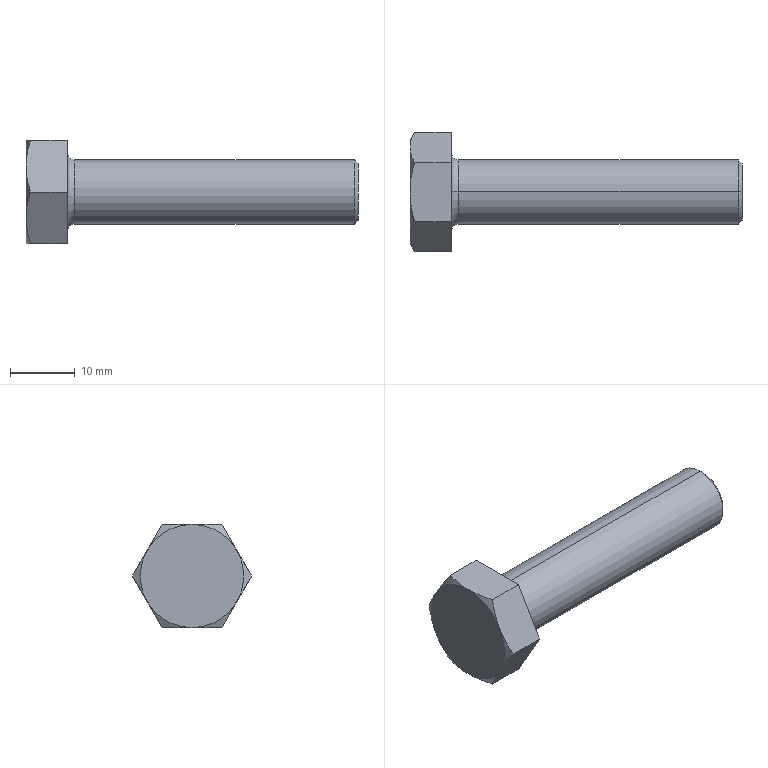Part | SolidWorks | features Chamfer 2, RevCut 2, Revolution 2, Extrusion 1, ICE 1 | 1 solid | 21 faces | box 51.4 x 18.475 x 16 mm | volume 4953 mm3 | plane 9 | cone 8 | cylinder 2 | torus 2 | commonest cylinder face diameters 10 x2
STEP:
#1=CARTESIAN_POINT('',(51.4,0.,-4.444));
#2=VERTEX_POINT('',#1);
#3=CARTESIAN_POINT('',(51.4,0.,4.444));
#4=VERTEX_POINT('',#3);
#5=CARTESIAN_POINT('',(51.4,0.,0.));
#6=DIRECTION('',(1.,0.,0.));
#7=DIRECTION('',(0.,0.,1.));
#8=AXIS2_PLACEMENT_3D('',#5,#6,#7);
#9=CIRCLE('',#8,4.444);
#10=EDGE_CURVE('',#2,#4,#9,.T.);
#11=ORIENTED_EDGE('',*,*,#10,.F.);
#12=CARTESIAN_POINT('',(50.844,0.,-5.));
#13=VERTEX_POINT('',#12);
#14=CARTESIAN_POINT('',(50.844,0.,-5.));
#15=DIRECTION('',(-0.7071,0.,-0.7071));
#16=VECTOR('',#15,1000.);
#17=LINE('',#14,#16);
#18=EDGE_CURVE('',#2,#13,#17,.T.);
#19=ORIENTED_EDGE('',*,*,#18,.T.);
#20=CARTESIAN_POINT('',(50.844,0.,5.));
#21=VERTEX_POINT('',#20);
#22=CARTESIAN_POINT('',(50.844,0.,0.));
#23=DIRECTION('',(-1.,0.,0.));
#24=DIRECTION('',(0.,0.,1.));
#25=AXIS2_PLACEMENT_3D('',#22,#23,#24);
#26=CIRCLE('',#25,5.);
#27=EDGE_CURVE('',#21,#13,#26,.T.);
#28=ORIENTED_EDGE('',*,*,#27,.F.);
#29=CARTESIAN_POINT('',(50.844,0.,5.));
#30=DIRECTION('',(-0.7071,0.,0.7071));
#31=VECTOR('',#30,1000.);
#32=LINE('',#29,#31);
#33=EDGE_CURVE('',#4,#21,#32,.T.);
#34=ORIENTED_EDGE('',*,*,#33,.F.);
#35=EDGE_LOOP('',(#11,#19,#28,#34));
#36=FACE_OUTER_BOUND('',#35,.T.);
#37=CARTESIAN_POINT('',(50.844,0.,0.));
#38=DIRECTION('',(-1.,0.,0.));
#39=DIRECTION('',(0.,0.,1.));
#40=AXIS2_PLACEMENT_3D('',#37,#38,#39);
#41=CONICAL_SURFACE('',#40,5.,0.7854);
#42=ADVANCED_FACE('',(#36),#41,.T.);
#43=ORIENTED_EDGE('',*,*,#27,.T.);
#44=CARTESIAN_POINT('',(7.5,0.,-5.));
#45=VERTEX_POINT('',#44);
#46=CARTESIAN_POINT('',(6.4,0.,-5.));
#47=DIRECTION('',(-1.,0.,0.));
#48=VECTOR('',#47,1000.);
#49=LINE('',#46,#48);
#50=EDGE_CURVE('',#13,#45,#49,.T.);
#51=ORIENTED_EDGE('',*,*,#50,.T.);
#52=CARTESIAN_POINT('',(7.5,0.,5.));
#53=VERTEX_POINT('',#52);
#54=CARTESIAN_POINT('',(7.5,0.,0.));
#55=DIRECTION('',(-1.,0.,0.));
#56=DIRECTION('',(0.,0.,1.));
#57=AXIS2_PLACEMENT_3D('',#54,#55,#56);
#58=CIRCLE('',#57,5.);
#59=EDGE_CURVE('',#53,#45,#58,.T.);
#60=ORIENTED_EDGE('',*,*,#59,.F.);
#61=CARTESIAN_POINT('',(6.4,0.,5.));
#62=DIRECTION('',(-1.,0.,0.));
#63=VECTOR('',#62,1000.);
#64=LINE('',#61,#63);
#65=EDGE_CURVE('',#21,#53,#64,.T.);
#66=ORIENTED_EDGE('',*,*,#65,.F.);
#67=EDGE_LOOP('',(#43,#51,#60,#66));
#68=FACE_OUTER_BOUND('',#67,.T.);
#69=CARTESIAN_POINT('',(6.4,0.,0.));
#70=DIRECTION('',(-1.,0.,0.));
#71=DIRECTION('',(0.,0.,1.));
#72=AXIS2_PLACEMENT_3D('',#69,#70,#71);
#73=CYLINDRICAL_SURFACE('',#72,5.);
#74=ADVANCED_FACE('',(#68),#73,.T.);
#75=CARTESIAN_POINT('',(6.4,0.,-6.1));
#76=VERTEX_POINT('',#75);
#77=CARTESIAN_POINT('',(6.4,0.,6.1));
#78=VERTEX_POINT('',#77);
#79=CARTESIAN_POINT('',(6.4,0.,0.));
#80=DIRECTION('',(-1.,0.,0.));
#81=DIRECTION('',(0.,0.,1.));
#82=AXIS2_PLACEMENT_3D('',#79,#80,#81);
#83=CIRCLE('',#82,6.1);
#84=EDGE_CURVE('',#76,#78,#83,.T.);
#85=ORIENTED_EDGE('',*,*,#84,.F.);
#86=CARTESIAN_POINT('',(7.5,0.,-6.1));
#87=DIRECTION('',(0.,1.,0.));
#88=DIRECTION('',(0.,0.,1.));
#89=AXIS2_PLACEMENT_3D('',#86,#87,#88);
#90=CIRCLE('',#89,1.1);
#91=EDGE_CURVE('',#76,#45,#90,.T.);
#92=ORIENTED_EDGE('',*,*,#91,.T.);
#93=CARTESIAN_POINT('',(7.5,0.,0.));
#94=DIRECTION('',(-1.,0.,0.));
#95=DIRECTION('',(0.,0.,1.));
#96=AXIS2_PLACEMENT_3D('',#93,#94,#95);
#97=CIRCLE('',#96,5.);
#98=EDGE_CURVE('',#45,#53,#97,.T.);
#99=ORIENTED_EDGE('',*,*,#98,.T.);
#100=CARTESIAN_POINT('',(7.5,0.,6.1));
#101=DIRECTION('',(0.,-1.,0.));
#102=DIRECTION('',(0.,0.,-1.));
#103=AXIS2_PLACEMENT_3D('',#100,#101,#102);
#104=CIRCLE('',#103,1.1);
#105=EDGE_CURVE('',#78,#53,#104,.T.);
#106=ORIENTED_EDGE('',*,*,#105,.F.);
#107=EDGE_LOOP('',(#85,#92,#99,#106));
#108=FACE_OUTER_BOUND('',#107,.T.);
#109=CARTESIAN_POINT('',(7.5,0.,0.));
#110=DIRECTION('',(-1.,0.,0.));
#111=DIRECTION('',(0.,0.,1.));
#112=AXIS2_PLACEMENT_3D('',#109,#110,#111);
#113=TOROIDAL_SURFACE('',#112,6.1,1.1);
#114=ADVANCED_FACE('',(#108),#113,.F.);
#115=CARTESIAN_POINT('',(6.4,-4.619,-8.));
#116=VERTEX_POINT('',#115);
#117=CARTESIAN_POINT('',(6.4,4.619,-8.));
#118=VERTEX_POINT('',#117);
#119=CARTESIAN_POINT('',(6.4,-4.619,-8.));
#120=DIRECTION('',(0.,1.,0.));
#121=VECTOR('',#120,1000.);
#122=LINE('',#119,#121);
#123=EDGE_CURVE('',#116,#118,#122,.T.);
#124=ORIENTED_EDGE('',*,*,#123,.T.);
#125=CARTESIAN_POINT('',(6.4,9.238,0.));
#126=VERTEX_POINT('',#125);
#127=CARTESIAN_POINT('',(6.4,4.619,-8.));
#128=DIRECTION('',(0.,0.5,0.866));
#129=VECTOR('',#128,1000.);
#130=LINE('',#127,#129);
#131=EDGE_CURVE('',#118,#126,#130,.T.);
#132=ORIENTED_EDGE('',*,*,#131,.T.);
#133=CARTESIAN_POINT('',(6.4,4.619,8.));
#134=VERTEX_POINT('',#133);
#135=CARTESIAN_POINT('',(6.4,9.238,0.));
#136=DIRECTION('',(0.,-0.5,0.866));
#137=VECTOR('',#136,1000.);
#138=LINE('',#135,#137);
#139=EDGE_CURVE('',#126,#134,#138,.T.);
#140=ORIENTED_EDGE('',*,*,#139,.T.);
#141=CARTESIAN_POINT('',(6.4,-4.619,8.));
#142=VERTEX_POINT('',#141);
#143=CARTESIAN_POINT('',(6.4,4.619,8.));
#144=DIRECTION('',(0.,-1.,0.));
#145=VECTOR('',#144,1000.);
#146=LINE('',#143,#145);
#147=EDGE_CURVE('',#134,#142,#146,.T.);
#148=ORIENTED_EDGE('',*,*,#147,.T.);
#149=CARTESIAN_POINT('',(6.4,-9.238,0.));
#150=VERTEX_POINT('',#149);
#151=CARTESIAN_POINT('',(6.4,-4.619,8.));
#152=DIRECTION('',(0.,-0.5,-0.866));
#153=VECTOR('',#152,1000.);
#154=LINE('',#151,#153);
#155=EDGE_CURVE('',#142,#150,#154,.T.);
#156=ORIENTED_EDGE('',*,*,#155,.T.);
#157=CARTESIAN_POINT('',(6.4,-9.238,0.));
#158=DIRECTION('',(0.,0.5,-0.866));
#159=VECTOR('',#158,1000.);
#160=LINE('',#157,#159);
#161=EDGE_CURVE('',#150,#116,#160,.T.);
#162=ORIENTED_EDGE('',*,*,#161,.T.);
#163=EDGE_LOOP('',(#124,#132,#140,#148,#156,#162));
#164=FACE_OUTER_BOUND('',#163,.T.);
#165=CARTESIAN_POINT('',(6.4,0.,0.));
#166=DIRECTION('',(-1.,0.,0.));
#167=DIRECTION('',(0.,0.,1.));
#168=AXIS2_PLACEMENT_3D('',#165,#166,#167);
#169=CIRCLE('',#168,6.1);
#170=EDGE_CURVE('',#78,#76,#169,.T.);
#171=ORIENTED_EDGE('',*,*,#170,.T.);
#172=ORIENTED_EDGE('',*,*,#84,.T.);
#173=EDGE_LOOP('',(#171,#172));
#174=FACE_BOUND('',#173,.T.);
#175=CARTESIAN_POINT('',(6.4,4.619,-8.));
#176=DIRECTION('',(1.,0.,0.));
#177=DIRECTION('',(0.,0.,-1.));
#178=AXIS2_PLACEMENT_3D('',#175,#176,#177);
#179=PLANE('',#178);
#180=ADVANCED_FACE('',(#164,#174),#179,.T.);
#181=CARTESIAN_POINT('',(0.7145,4.619,-8.));
#182=VERTEX_POINT('',#181);
#183=CARTESIAN_POINT('',(0.,0.,-8.));
#184=VERTEX_POINT('',#183);
#185=CARTESIAN_POINT('',(0.7145,4.619,-8.));
#186=CARTESIAN_POINT('',(0.4989,3.872,-8.));
#187=CARTESIAN_POINT('',(0.3194,3.115,-8.));
#188=CARTESIAN_POINT('',(0.06895,1.573,-8.));
#189=CARTESIAN_POINT('',(0.,0.781,-8.));
#190=CARTESIAN_POINT('',(0.,0.,-8.));
#191=B_SPLINE_CURVE_WITH_KNOTS('',3,(#185,#186,#187,#188,#189,#190),.UNSPECIFIED.,.F.,.F.,(4,2,4),(0.003372,0.005703,0.008035),.UNSPECIFIED.);
#192=EDGE_CURVE('',#182,#184,#191,.T.);
#193=ORIENTED_EDGE('',*,*,#192,.F.);
#194=CARTESIAN_POINT('',(6.4,4.619,-8.));
#195=DIRECTION('',(-1.,0.,0.));
#196=VECTOR('',#195,1000.);
#197=LINE('',#194,#196);
#198=EDGE_CURVE('',#118,#182,#197,.T.);
#199=ORIENTED_EDGE('',*,*,#198,.F.);
#200=ORIENTED_EDGE('',*,*,#123,.F.);
#201=CARTESIAN_POINT('',(0.7145,-4.619,-8.));
#202=VERTEX_POINT('',#201);
#203=CARTESIAN_POINT('',(6.4,-4.619,-8.));
#204=DIRECTION('',(-1.,0.,0.));
#205=VECTOR('',#204,1000.);
#206=LINE('',#203,#205);
#207=EDGE_CURVE('',#116,#202,#206,.T.);
#208=ORIENTED_EDGE('',*,*,#207,.T.);
#209=CARTESIAN_POINT('',(0.,0.,-8.));
#210=CARTESIAN_POINT('',(0.,-0.7805,-8.));
#211=CARTESIAN_POINT('',(0.06709,-1.556,-8.));
#212=CARTESIAN_POINT('',(0.3158,-3.098,-8.));
#213=CARTESIAN_POINT('',(0.4977,-3.868,-8.));
#214=CARTESIAN_POINT('',(0.7145,-4.619,-8.));
#215=B_SPLINE_CURVE_WITH_KNOTS('',3,(#209,#210,#211,#212,#213,#214),.UNSPECIFIED.,.F.,.F.,(4,2,4),(0.008035,0.01037,0.0127),.UNSPECIFIED.);
#216=EDGE_CURVE('',#184,#202,#215,.T.);
#217=ORIENTED_EDGE('',*,*,#216,.F.);
#218=EDGE_LOOP('',(#193,#199,#200,#208,#217));
#219=FACE_OUTER_BOUND('',#218,.T.);
#220=CARTESIAN_POINT('',(6.4,-4.619,-8.));
#221=DIRECTION('',(0.,0.,1.));
#222=DIRECTION('',(1.,0.,0.));
#223=AXIS2_PLACEMENT_3D('',#220,#221,#222);
#224=PLANE('',#223);
#225=ADVANCED_FACE('',(#219),#224,.F.);
#226=CARTESIAN_POINT('',(0.7145,9.238,0.));
#227=VERTEX_POINT('',#226);
#228=CARTESIAN_POINT('',(0.,6.928,-4.));
#229=VERTEX_POINT('',#228);
#230=CARTESIAN_POINT('',(0.7145,9.238,0.));
#231=CARTESIAN_POINT('',(0.4964,8.86,-0.6543));
#232=CARTESIAN_POINT('',(0.3167,8.479,-1.313));
#233=CARTESIAN_POINT('',(0.0681,7.71,-2.646));
#234=CARTESIAN_POINT('',(0.,7.322,-3.319));
#235=CARTESIAN_POINT('',(0.,6.928,-4.));
#236=B_SPLINE_CURVE_WITH_KNOTS('',3,(#230,#231,#232,#233,#234,#235),.UNSPECIFIED.,.F.,.F.,(4,2,4),(0.000000238,0.002337,0.004674),.UNSPECIFIED.);
#237=EDGE_CURVE('',#227,#229,#236,.T.);
#238=ORIENTED_EDGE('',*,*,#237,.F.);
#239=CARTESIAN_POINT('',(6.4,9.238,0.));
#240=DIRECTION('',(-1.,0.,0.));
#241=VECTOR('',#240,1000.);
#242=LINE('',#239,#241);
#243=EDGE_CURVE('',#126,#227,#242,.T.);
#244=ORIENTED_EDGE('',*,*,#243,.F.);
#245=ORIENTED_EDGE('',*,*,#131,.F.);
#246=ORIENTED_EDGE('',*,*,#198,.T.);
#247=CARTESIAN_POINT('',(0.,6.928,-4.));
#248=CARTESIAN_POINT('',(0.,6.732,-4.339));
#249=CARTESIAN_POINT('',(0.01689,6.535,-4.68));
#250=CARTESIAN_POINT('',(0.08225,6.146,-5.355));
#251=CARTESIAN_POINT('',(0.1307,5.952,-5.69));
#252=CARTESIAN_POINT('',(0.3174,5.376,-6.689));
#253=CARTESIAN_POINT('',(0.497,4.996,-7.347));
#254=CARTESIAN_POINT('',(0.7145,4.619,-8.));
#255=B_SPLINE_CURVE_WITH_KNOTS('',3,(#247,#248,#249,#250,#251,#252,#253,#254),.UNSPECIFIED.,.F.,.F.,(4,2,2,4),(0.004674,0.005838,0.007002,0.00933),.UNSPECIFIED.);
#256=EDGE_CURVE('',#229,#182,#255,.T.);
#257=ORIENTED_EDGE('',*,*,#256,.F.);
#258=EDGE_LOOP('',(#238,#244,#245,#246,#257));
#259=FACE_OUTER_BOUND('',#258,.T.);
#260=CARTESIAN_POINT('',(6.4,4.619,-8.));
#261=DIRECTION('',(0.,-0.866,0.5));
#262=DIRECTION('',(0.,-0.5,-0.866));
#263=AXIS2_PLACEMENT_3D('',#260,#261,#262);
#264=PLANE('',#263);
#265=ADVANCED_FACE('',(#259),#264,.F.);
#266=CARTESIAN_POINT('',(0.7145,4.619,8.));
#267=VERTEX_POINT('',#266);
#268=CARTESIAN_POINT('',(0.,6.928,4.));
#269=VERTEX_POINT('',#268);
#270=CARTESIAN_POINT('',(0.7145,4.619,8.));
#271=CARTESIAN_POINT('',(0.4964,4.997,7.346));
#272=CARTESIAN_POINT('',(0.3167,5.377,6.687));
#273=CARTESIAN_POINT('',(0.0681,6.146,5.354));
#274=CARTESIAN_POINT('',(0.,6.535,4.681));
#275=CARTESIAN_POINT('',(0.,6.928,4.));
#276=B_SPLINE_CURVE_WITH_KNOTS('',3,(#270,#271,#272,#273,#274,#275),.UNSPECIFIED.,.F.,.F.,(4,2,4),(0.000000238,0.002337,0.004674),.UNSPECIFIED.);
#277=EDGE_CURVE('',#267,#269,#276,.T.);
#278=ORIENTED_EDGE('',*,*,#277,.F.);
#279=CARTESIAN_POINT('',(6.4,4.619,8.));
#280=DIRECTION('',(-1.,0.,0.));
#281=VECTOR('',#280,1000.);
#282=LINE('',#279,#281);
#283=EDGE_CURVE('',#134,#267,#282,.T.);
#284=ORIENTED_EDGE('',*,*,#283,.F.);
#285=ORIENTED_EDGE('',*,*,#139,.F.);
#286=ORIENTED_EDGE('',*,*,#243,.T.);
#287=CARTESIAN_POINT('',(0.,6.928,4.));
#288=CARTESIAN_POINT('',(0.,7.124,3.661));
#289=CARTESIAN_POINT('',(0.01689,7.321,3.32));
#290=CARTESIAN_POINT('',(0.08225,7.711,2.645));
#291=CARTESIAN_POINT('',(0.1307,7.904,2.31));
#292=CARTESIAN_POINT('',(0.3174,8.481,1.311));
#293=CARTESIAN_POINT('',(0.497,8.861,0.6527));
#294=CARTESIAN_POINT('',(0.7145,9.238,0.));
#295=B_SPLINE_CURVE_WITH_KNOTS('',3,(#287,#288,#289,#290,#291,#292,#293,#294),.UNSPECIFIED.,.F.,.F.,(4,2,2,4),(0.004674,0.005838,0.007002,0.00933),.UNSPECIFIED.);
#296=EDGE_CURVE('',#269,#227,#295,.T.);
#297=ORIENTED_EDGE('',*,*,#296,.F.);
#298=EDGE_LOOP('',(#278,#284,#285,#286,#297));
#299=FACE_OUTER_BOUND('',#298,.T.);
#300=CARTESIAN_POINT('',(6.4,9.238,0.));
#301=DIRECTION('',(0.,-0.866,-0.5));
#302=DIRECTION('',(0.,0.5,-0.866));
#303=AXIS2_PLACEMENT_3D('',#300,#301,#302);
#304=PLANE('',#303);
#305=ADVANCED_FACE('',(#299),#304,.F.);
#306=CARTESIAN_POINT('',(0.7145,-4.619,8.));
#307=VERTEX_POINT('',#306);
#308=CARTESIAN_POINT('',(0.,0.,8.));
#309=VERTEX_POINT('',#308);
#310=CARTESIAN_POINT('',(0.7145,-4.619,8.));
#311=CARTESIAN_POINT('',(0.4977,-3.868,8.));
#312=CARTESIAN_POINT('',(0.3158,-3.098,8.));
#313=CARTESIAN_POINT('',(0.06709,-1.556,8.));
#314=CARTESIAN_POINT('',(0.,-0.7805,8.));
#315=CARTESIAN_POINT('',(0.,0.,8.));
#316=B_SPLINE_CURVE_WITH_KNOTS('',3,(#310,#311,#312,#313,#314,#315),.UNSPECIFIED.,.F.,.F.,(4,2,4),(0.008254,0.01059,0.01293),.UNSPECIFIED.);
#317=EDGE_CURVE('',#307,#309,#316,.T.);
#318=ORIENTED_EDGE('',*,*,#317,.F.);
#319=CARTESIAN_POINT('',(6.4,-4.619,8.));
#320=DIRECTION('',(-1.,0.,0.));
#321=VECTOR('',#320,1000.);
#322=LINE('',#319,#321);
#323=EDGE_CURVE('',#142,#307,#322,.T.);
#324=ORIENTED_EDGE('',*,*,#323,.F.);
#325=ORIENTED_EDGE('',*,*,#147,.F.);
#326=ORIENTED_EDGE('',*,*,#283,.T.);
#327=CARTESIAN_POINT('',(0.,0.,8.));
#328=CARTESIAN_POINT('',(0.,0.781,8.));
#329=CARTESIAN_POINT('',(0.06895,1.573,8.));
#330=CARTESIAN_POINT('',(0.3194,3.115,8.));
#331=CARTESIAN_POINT('',(0.4989,3.872,8.));
#332=CARTESIAN_POINT('',(0.7145,4.619,8.));
#333=B_SPLINE_CURVE_WITH_KNOTS('',3,(#327,#328,#329,#330,#331,#332),.UNSPECIFIED.,.F.,.F.,(4,2,4),(0.01293,0.01526,0.0176),.UNSPECIFIED.);
#334=EDGE_CURVE('',#309,#267,#333,.T.);
#335=ORIENTED_EDGE('',*,*,#334,.F.);
#336=EDGE_LOOP('',(#318,#324,#325,#326,#335));
#337=FACE_OUTER_BOUND('',#336,.T.);
#338=CARTESIAN_POINT('',(6.4,4.619,8.));
#339=DIRECTION('',(0.,0.,-1.));
#340=DIRECTION('',(0.,1.,0.));
#341=AXIS2_PLACEMENT_3D('',#338,#339,#340);
#342=PLANE('',#341);
#343=ADVANCED_FACE('',(#337),#342,.F.);
#344=CARTESIAN_POINT('',(0.7145,-9.238,0.));
#345=VERTEX_POINT('',#344);
#346=CARTESIAN_POINT('',(0.,-6.928,4.));
#347=VERTEX_POINT('',#346);
#348=CARTESIAN_POINT('',(0.7145,-9.238,0.));
#349=CARTESIAN_POINT('',(0.4964,-8.86,0.6543));
#350=CARTESIAN_POINT('',(0.3167,-8.479,1.313));
#351=CARTESIAN_POINT('',(0.0681,-7.71,2.646));
#352=CARTESIAN_POINT('',(0.,-7.322,3.319));
#353=CARTESIAN_POINT('',(0.,-6.928,4.));
#354=B_SPLINE_CURVE_WITH_KNOTS('',3,(#348,#349,#350,#351,#352,#353),.UNSPECIFIED.,.F.,.F.,(4,2,4),(0.000000238,0.002337,0.004674),.UNSPECIFIED.);
#355=EDGE_CURVE('',#345,#347,#354,.T.);
#356=ORIENTED_EDGE('',*,*,#355,.F.);
#357=CARTESIAN_POINT('',(6.4,-9.238,0.));
#358=DIRECTION('',(-1.,0.,0.));
#359=VECTOR('',#358,1000.);
#360=LINE('',#357,#359);
#361=EDGE_CURVE('',#150,#345,#360,.T.);
#362=ORIENTED_EDGE('',*,*,#361,.F.);
#363=ORIENTED_EDGE('',*,*,#155,.F.);
#364=ORIENTED_EDGE('',*,*,#323,.T.);
#365=CARTESIAN_POINT('',(0.,-6.928,4.));
#366=CARTESIAN_POINT('',(0.,-6.732,4.339));
#367=CARTESIAN_POINT('',(0.01689,-6.535,4.68));
#368=CARTESIAN_POINT('',(0.08225,-6.146,5.355));
#369=CARTESIAN_POINT('',(0.1307,-5.952,5.69));
#370=CARTESIAN_POINT('',(0.3174,-5.376,6.689));
#371=CARTESIAN_POINT('',(0.497,-4.996,7.347));
#372=CARTESIAN_POINT('',(0.7145,-4.619,8.));
#373=B_SPLINE_CURVE_WITH_KNOTS('',3,(#365,#366,#367,#368,#369,#370,#371,#372),.UNSPECIFIED.,.F.,.F.,(4,2,2,4),(0.004674,0.005838,0.007002,0.00933),.UNSPECIFIED.);
#374=EDGE_CURVE('',#347,#307,#373,.T.);
#375=ORIENTED_EDGE('',*,*,#374,.F.);
#376=EDGE_LOOP('',(#356,#362,#363,#364,#375));
#377=FACE_OUTER_BOUND('',#376,.T.);
#378=CARTESIAN_POINT('',(6.4,-4.619,8.));
#379=DIRECTION('',(0.,0.866,-0.5));
#380=DIRECTION('',(0.,0.5,0.866));
#381=AXIS2_PLACEMENT_3D('',#378,#379,#380);
#382=PLANE('',#381);
#383=ADVANCED_FACE('',(#377),#382,.F.);
#384=CARTESIAN_POINT('',(0.,-6.928,-4.));
#385=VERTEX_POINT('',#384);
#386=CARTESIAN_POINT('',(0.7145,-4.619,-8.));
#387=CARTESIAN_POINT('',(0.4964,-4.997,-7.346));
#388=CARTESIAN_POINT('',(0.3167,-5.377,-6.687));
#389=CARTESIAN_POINT('',(0.0681,-6.146,-5.354));
#390=CARTESIAN_POINT('',(0.,-6.535,-4.681));
#391=CARTESIAN_POINT('',(0.,-6.928,-4.));
#392=B_SPLINE_CURVE_WITH_KNOTS('',3,(#386,#387,#388,#389,#390,#391),.UNSPECIFIED.,.F.,.F.,(4,2,4),(0.000000238,0.002337,0.004674),.UNSPECIFIED.);
#393=EDGE_CURVE('',#202,#385,#392,.T.);
#394=ORIENTED_EDGE('',*,*,#393,.F.);
#395=ORIENTED_EDGE('',*,*,#207,.F.);
#396=ORIENTED_EDGE('',*,*,#161,.F.);
#397=ORIENTED_EDGE('',*,*,#361,.T.);
#398=CARTESIAN_POINT('',(0.,-6.928,-4.));
#399=CARTESIAN_POINT('',(0.,-7.124,-3.661));
#400=CARTESIAN_POINT('',(0.01689,-7.321,-3.32));
#401=CARTESIAN_POINT('',(0.08225,-7.711,-2.645));
#402=CARTESIAN_POINT('',(0.1307,-7.904,-2.31));
#403=CARTESIAN_POINT('',(0.3174,-8.481,-1.311));
#404=CARTESIAN_POINT('',(0.497,-8.861,-0.6527));
#405=CARTESIAN_POINT('',(0.7145,-9.238,0.));
#406=B_SPLINE_CURVE_WITH_KNOTS('',3,(#398,#399,#400,#401,#402,#403,#404,#405),.UNSPECIFIED.,.F.,.F.,(4,2,2,4),(0.004674,0.005838,0.007002,0.00933),.UNSPECIFIED.);
#407=EDGE_CURVE('',#385,#345,#406,.T.);
#408=ORIENTED_EDGE('',*,*,#407,.F.);
#409=EDGE_LOOP('',(#394,#395,#396,#397,#408));
#410=FACE_OUTER_BOUND('',#409,.T.);
#411=CARTESIAN_POINT('',(6.4,-9.238,0.));
#412=DIRECTION('',(0.,0.866,0.5));
#413=DIRECTION('',(0.,-0.5,0.866));
#414=AXIS2_PLACEMENT_3D('',#411,#412,#413);
#415=PLANE('',#414);
#416=ADVANCED_FACE('',(#410),#415,.F.);
#417=ORIENTED_EDGE('',*,*,#216,.T.);
#418=ORIENTED_EDGE('',*,*,#393,.T.);
#419=CARTESIAN_POINT('',(0.,0.,0.));
#420=DIRECTION('',(1.,0.,0.));
#421=DIRECTION('',(0.,0.,-1.));
#422=AXIS2_PLACEMENT_3D('',#419,#420,#421);
#423=CIRCLE('',#422,8.);
#424=EDGE_CURVE('',#385,#184,#423,.T.);
#425=ORIENTED_EDGE('',*,*,#424,.T.);
#426=EDGE_LOOP('',(#417,#418,#425));
#427=FACE_OUTER_BOUND('',#426,.T.);
#428=CARTESIAN_POINT('',(0.,0.,0.));
#429=DIRECTION('',(1.,0.,0.));
#430=DIRECTION('',(0.,0.,1.));
#431=AXIS2_PLACEMENT_3D('',#428,#429,#430);
#432=CONICAL_SURFACE('',#431,8.,1.047);
#433=ADVANCED_FACE('',(#427),#432,.T.);
#434=ORIENTED_EDGE('',*,*,#355,.T.);
#435=CARTESIAN_POINT('',(0.,0.,0.));
#436=DIRECTION('',(1.,0.,0.));
#437=DIRECTION('',(0.,0.,-1.));
#438=AXIS2_PLACEMENT_3D('',#435,#436,#437);
#439=CIRCLE('',#438,8.);
#440=EDGE_CURVE('',#347,#385,#439,.T.);
#441=ORIENTED_EDGE('',*,*,#440,.T.);
#442=ORIENTED_EDGE('',*,*,#407,.T.);
#443=EDGE_LOOP('',(#434,#441,#442));
#444=FACE_OUTER_BOUND('',#443,.T.);
#445=CARTESIAN_POINT('',(0.,0.,0.));
#446=DIRECTION('',(1.,0.,0.));
#447=DIRECTION('',(0.,0.,1.));
#448=AXIS2_PLACEMENT_3D('',#445,#446,#447);
#449=CONICAL_SURFACE('',#448,8.,1.047);
#450=ADVANCED_FACE('',(#444),#449,.T.);
#451=ORIENTED_EDGE('',*,*,#317,.T.);
#452=CARTESIAN_POINT('',(0.,0.,0.));
#453=DIRECTION('',(1.,0.,0.));
#454=DIRECTION('',(0.,0.,-1.));
#455=AXIS2_PLACEMENT_3D('',#452,#453,#454);
#456=CIRCLE('',#455,8.);
#457=EDGE_CURVE('',#309,#347,#456,.T.);
#458=ORIENTED_EDGE('',*,*,#457,.T.);
#459=ORIENTED_EDGE('',*,*,#374,.T.);
#460=EDGE_LOOP('',(#451,#458,#459));
#461=FACE_OUTER_BOUND('',#460,.T.);
#462=CARTESIAN_POINT('',(0.,0.,0.));
#463=DIRECTION('',(1.,0.,0.));
#464=DIRECTION('',(0.,0.,1.));
#465=AXIS2_PLACEMENT_3D('',#462,#463,#464);
#466=CONICAL_SURFACE('',#465,8.,1.047);
#467=ADVANCED_FACE('',(#461),#466,.T.);
#468=ORIENTED_EDGE('',*,*,#277,.T.);
#469=CARTESIAN_POINT('',(0.,0.,0.));
#470=DIRECTION('',(-1.,0.,0.));
#471=DIRECTION('',(0.,0.,1.));
#472=AXIS2_PLACEMENT_3D('',#469,#470,#471);
#473=CIRCLE('',#472,8.);
#474=EDGE_CURVE('',#309,#269,#473,.T.);
#475=ORIENTED_EDGE('',*,*,#474,.F.);
#476=ORIENTED_EDGE('',*,*,#334,.T.);
#477=EDGE_LOOP('',(#468,#475,#476));
#478=FACE_OUTER_BOUND('',#477,.T.);
#479=CARTESIAN_POINT('',(0.,0.,0.));
#480=DIRECTION('',(1.,0.,0.));
#481=DIRECTION('',(0.,0.,1.));
#482=AXIS2_PLACEMENT_3D('',#479,#480,#481);
#483=CONICAL_SURFACE('',#482,8.,1.047);
#484=ADVANCED_FACE('',(#478),#483,.T.);
#485=ORIENTED_EDGE('',*,*,#296,.T.);
#486=ORIENTED_EDGE('',*,*,#237,.T.);
#487=CARTESIAN_POINT('',(0.,0.,0.));
#488=DIRECTION('',(1.,0.,0.));
#489=DIRECTION('',(0.,0.,-1.));
#490=AXIS2_PLACEMENT_3D('',#487,#488,#489);
#491=CIRCLE('',#490,8.);
#492=EDGE_CURVE('',#229,#269,#491,.T.);
#493=ORIENTED_EDGE('',*,*,#492,.T.);
#494=EDGE_LOOP('',(#485,#486,#493));
#495=FACE_OUTER_BOUND('',#494,.T.);
#496=CARTESIAN_POINT('',(0.,0.,0.));
#497=DIRECTION('',(1.,0.,0.));
#498=DIRECTION('',(0.,0.,1.));
#499=AXIS2_PLACEMENT_3D('',#496,#497,#498);
#500=CONICAL_SURFACE('',#499,8.,1.047);
#501=ADVANCED_FACE('',(#495),#500,.T.);
#502=ORIENTED_EDGE('',*,*,#256,.T.);
#503=ORIENTED_EDGE('',*,*,#192,.T.);
#504=CARTESIAN_POINT('',(0.,0.,0.));
#505=DIRECTION('',(1.,0.,0.));
#506=DIRECTION('',(0.,0.,-1.));
#507=AXIS2_PLACEMENT_3D('',#504,#505,#506);
#508=CIRCLE('',#507,8.);
#509=EDGE_CURVE('',#184,#229,#508,.T.);
#510=ORIENTED_EDGE('',*,*,#509,.T.);
#511=EDGE_LOOP('',(#502,#503,#510));
#512=FACE_OUTER_BOUND('',#511,.T.);
#513=CARTESIAN_POINT('',(0.,0.,0.));
#514=DIRECTION('',(1.,0.,0.));
#515=DIRECTION('',(0.,0.,1.));
#516=AXIS2_PLACEMENT_3D('',#513,#514,#515);
#517=CONICAL_SURFACE('',#516,8.,1.047);
#518=ADVANCED_FACE('',(#512),#517,.T.);
#519=ORIENTED_EDGE('',*,*,#509,.F.);
#520=ORIENTED_EDGE('',*,*,#424,.F.);
#521=ORIENTED_EDGE('',*,*,#440,.F.);
#522=ORIENTED_EDGE('',*,*,#457,.F.);
#523=ORIENTED_EDGE('',*,*,#474,.T.);
#524=ORIENTED_EDGE('',*,*,#492,.F.);
#525=EDGE_LOOP('',(#519,#520,#521,#522,#523,#524));
#526=FACE_OUTER_BOUND('',#525,.T.);
#527=CARTESIAN_POINT('',(0.,4.619,-8.));
#528=DIRECTION('',(1.,0.,0.));
#529=DIRECTION('',(0.,0.,-1.));
#530=AXIS2_PLACEMENT_3D('',#527,#528,#529);
#531=PLANE('',#530);
#532=ADVANCED_FACE('',(#526),#531,.F.);
#533=ORIENTED_EDGE('',*,*,#91,.F.);
#534=ORIENTED_EDGE('',*,*,#170,.F.);
#535=ORIENTED_EDGE('',*,*,#105,.T.);
#536=ORIENTED_EDGE('',*,*,#59,.T.);
#537=EDGE_LOOP('',(#533,#534,#535,#536));
#538=FACE_OUTER_BOUND('',#537,.T.);
#539=CARTESIAN_POINT('',(7.5,0.,0.));
#540=DIRECTION('',(-1.,0.,0.));
#541=DIRECTION('',(0.,0.,1.));
#542=AXIS2_PLACEMENT_3D('',#539,#540,#541);
#543=TOROIDAL_SURFACE('',#542,6.1,1.1);
#544=ADVANCED_FACE('',(#538),#543,.F.);
#545=CARTESIAN_POINT('',(51.4,0.,0.));
#546=DIRECTION('',(1.,0.,0.));
#547=DIRECTION('',(0.,0.,1.));
#548=AXIS2_PLACEMENT_3D('',#545,#546,#547);
#549=CIRCLE('',#548,4.444);
#550=EDGE_CURVE('',#4,#2,#549,.T.);
#551=ORIENTED_EDGE('',*,*,#550,.T.);
#552=ORIENTED_EDGE('',*,*,#10,.T.);
#553=EDGE_LOOP('',(#551,#552));
#554=FACE_OUTER_BOUND('',#553,.T.);
#555=CARTESIAN_POINT('',(51.4,5.,0.));
#556=DIRECTION('',(-1.,0.,0.));
#557=DIRECTION('',(0.,0.,1.));
#558=AXIS2_PLACEMENT_3D('',#555,#556,#557);
#559=PLANE('',#558);
#560=ADVANCED_FACE('',(#554),#559,.F.);
#561=ORIENTED_EDGE('',*,*,#50,.F.);
#562=CARTESIAN_POINT('',(50.844,0.,0.));
#563=DIRECTION('',(-1.,0.,0.));
#564=DIRECTION('',(0.,0.,1.));
#565=AXIS2_PLACEMENT_3D('',#562,#563,#564);
#566=CIRCLE('',#565,5.);
#567=EDGE_CURVE('',#13,#21,#566,.T.);
#568=ORIENTED_EDGE('',*,*,#567,.T.);
#569=ORIENTED_EDGE('',*,*,#65,.T.);
#570=ORIENTED_EDGE('',*,*,#98,.F.);
#571=EDGE_LOOP('',(#561,#568,#569,#570));
#572=FACE_OUTER_BOUND('',#571,.T.);
#573=CARTESIAN_POINT('',(6.4,0.,0.));
#574=DIRECTION('',(-1.,0.,0.));
#575=DIRECTION('',(0.,0.,1.));
#576=AXIS2_PLACEMENT_3D('',#573,#574,#575);
#577=CYLINDRICAL_SURFACE('',#576,5.);
#578=ADVANCED_FACE('',(#572),#577,.T.);
#579=ORIENTED_EDGE('',*,*,#18,.F.);
#580=ORIENTED_EDGE('',*,*,#550,.F.);
#581=ORIENTED_EDGE('',*,*,#33,.T.);
#582=ORIENTED_EDGE('',*,*,#567,.F.);
#583=EDGE_LOOP('',(#579,#580,#581,#582));
#584=FACE_OUTER_BOUND('',#583,.T.);
#585=CARTESIAN_POINT('',(50.844,0.,0.));
#586=DIRECTION('',(-1.,0.,0.));
#587=DIRECTION('',(0.,0.,1.));
#588=AXIS2_PLACEMENT_3D('',#585,#586,#587);
#589=CONICAL_SURFACE('',#588,5.,0.7854);
#590=ADVANCED_FACE('',(#584),#589,.T.);
#591=CLOSED_SHELL('',(#42,#74,#114,#180,#225,#265,#305,#343,#383,#416,#433,#450,#467,#484,#501,#518,#532,#544,#560,#578,#590));
#592=MANIFOLD_SOLID_BREP('',#591);
#593=CARTESIAN_POINT('',(0.,0.,0.));
#594=DIRECTION('',(0.,0.,1.));
#595=DIRECTION('',(1.,0.,0.));
#596=AXIS2_PLACEMENT_3D('',#593,#594,#595);
#597=(LENGTH_UNIT()NAMED_UNIT(*)SI_UNIT(.MILLI.,.METRE.));
#598=UNCERTAINTY_MEASURE_WITH_UNIT(LENGTH_MEASURE(0.00001),#597,'','');
#599=(NAMED_UNIT(*)PLANE_ANGLE_UNIT()SI_UNIT($,.RADIAN.));
#600=(NAMED_UNIT(*)SI_UNIT($,.STERADIAN.)SOLID_ANGLE_UNIT());
#601=(GEOMETRIC_REPRESENTATION_CONTEXT(3)GLOBAL_UNCERTAINTY_ASSIGNED_CONTEXT((#598))GLOBAL_UNIT_ASSIGNED_CONTEXT((#597,#599,#600))REPRESENTATION_CONTEXT('',''));
#602=ADVANCED_BREP_SHAPE_REPRESENTATION('',(#592,#596),#601);